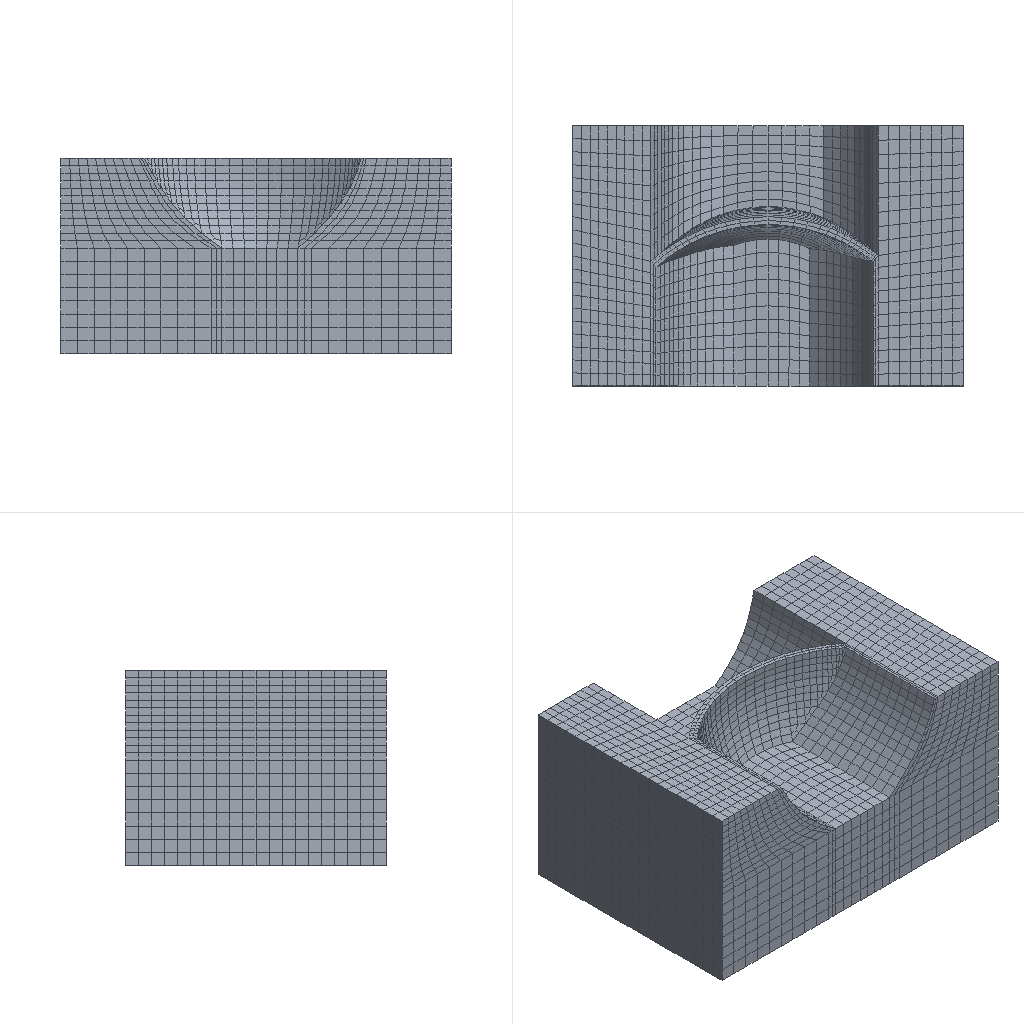Simulation study | abaqus
Set-up summary:
category,name,step,type,value,unit,region
solver,abaqus
solver,version,,,Abaqus/Standard 2020
units,not stated in the deck,,not stated
analysis,deck,,static,static
load_step,Step-2,Step-2,static
load_step,requested,,,1
mesh,nodes,,,11349
mesh,elements,,,9392
element_type,C3D8RP,,solid,9392
load,load commands in deck,,count,275
bc,support commands in deck,,count,1
material,MAT-BAJI,,in results
material,MAT-BATI,,in results
check,setup vs results,,match,"per instance, exact: element labels, types and connectivity; labels of the nodes the elements use; coordinates of those nodes at SINGLE_PRECISION in 1 of 1 instance(s)"
Abaqus input file, long lists of numbers shortened:
*Heading
** Job name: Job-2 Model name: model-mesh-Copy
** Generated by: Abaqus/CAE 2020
*Preprint, echo=NO, model=NO, history=NO, contact=NO
**
** PARTS
**
*Part, name=Part-10
*Node
      1,  -79.508,  -35.548,         57.5
      2,  -80.694,  -34.215,          69.
** (11347 more lines like these left out)
*Element, type=C3D8RP
1, 1819,  221, 1818, 6648,  219,    1,  220, 1817
2, 1818,  223, 1820, 6648,  220,    2,  222, 1817
** (9390 more lines like these left out)
*Nset, nset=bati
     1,     2,     3,     4,     5,     6,     7,     8,     9,    10,    11,    12,    13,    14,    15,    16
    17,    18,    19,    20,    21,    22,    23,    24,    25,    26,    27,    28,    29,    30,    31,    32
** (49 more lines like these left out)
*Elset, elset=bati
    1,    2,    3,    4,    5,    6,    7,    8,    9,   10,   11,   12,   13,   14,   15,   16
   17,   18,   19,   20,   21,   22,   23,   24,   25,   26,   27,   28,   29,   30,   31,   32
** (28 more lines like these left out)
*Nset, nset=baji
     1,     3,     5,     6,    15,    16,    26,    27,    38,    39,    52,    53,    68,    69,    70,    71
    72,    74,    75,    77,    98,    99,   108,   109,   117,   118,   121,   124,   127,   128,   129,   130
** (663 more lines like these left out)
*Elset, elset=baji, generate
  469,  9380,     1
** Section: Sec-bati
*Solid Section, elset=bati, material=Mat-bati
,
** Section: Sec-baji
*Solid Section, elset=baji, material=Mat-baji
,
*End Part
**
*Part, name=crack
*End Part
**
**
** ASSEMBLY
**
*Assembly, name=Assembly
**
*Instance, name=Part-10-1, part=Part-10
*End Instance
**
*Instance, name=crack-1, part=crack
23.198,       4.068, 38.045
23.198,       4.068, 38.045, 23.198, 5.068, 38.045, 80.
*End Instance
**
*Nset, nset=Set-9, instance=Part-10-1
    4,    5,    6,    7,   10,   11,   14,   15,   17,   20,   21,   23,   24,   26,   29,   30
   33,   34,   37,   38,   40,   42,   45,   46,   48,   50,   52,   55,   56,   59,   60,   63
** (15 more lines like these left out)
*Elset, elset=Set-9, instance=Part-10-1
    4,    5,    6,    7,    9,   11,   13,   16,   18,   20,   22,   23,   24,   25,   29,   31
   33,   35,   37,   39,   41,   43,   45,   47,   49,   51,   53,   54,   55,   59,   61,   63
** (13 more lines like these left out)
*Nset, nset=Set-10, instance=Part-10-1
    1,    2,    3,    4,    6,    8,    9,   10,   12,   13,   14,   16,   18,   19,   22,   25
   27,   28,   29,   31,   32,   33,   35,   36,   39,   41,   43,   44,   47,   49,   51,   53
** (19 more lines like these left out)
*Elset, elset=Set-10, instance=Part-10-1
    1,    2,    3,    4,    6,    8,    9,   10,   12,   13,   14,   15,   17,   19,   20,   21
   22,   26,   27,   28,   30,   32,   34,   36,   38,   40,   42,   44,   46,   48,   50,   52
** (15 more lines like these left out)
*Nset, nset=Set-11, instance=Part-10-1
     1,     2,     3,     4,     5,     6,     7,     8,     9,    10,    11,    12,    13,    14,    15,    16
    17,    18,    19,    20,    21,    22,    23,    24,    25,    26,    27,    28,    29,    30,    31,    32
** (49 more lines like these left out)
*Elset, elset=Set-11, instance=Part-10-1
    1,    2,    3,    4,    5,    6,    7,    8,    9,   10,   11,   12,   13,   14,   15,   16
   17,   18,   19,   20,   21,   22,   23,   24,   25,   26,   27,   28,   29,   30,   31,   32
** (34 more lines like these left out)
*Nset, nset=Set-14, instance=Part-10-1
  131,  132,  133,  134,  136,  137,  138,  139,  140,  142,  143,  145,  146,  150,  152,  154
  157,  158,  576,  577,  578,  579,  580,  581,  582,  583,  584,  585,  586,  587,  588,  589
** (35 more lines like these left out)
*Elset, elset=Set-14, instance=Part-10-1
  700,  701,  702,  703,  704,  705,  706,  707,  708,  709,  710,  711,  712,  713,  714,  715
  716,  717,  718,  719,  720,  721,  722,  723,  724,  725,  726,  727,  728,  729,  730,  731
** (32 more lines like these left out)
*Nset, nset=Set-15, instance=Part-10-1
    4,    5,    6,    7,   10,   11,   14,   15,   17,   20,   21,   23,   24,   26,   29,   30
   33,   34,   37,   38,   40,   42,   45,   46,   48,   50,   52,   55,   56,   59,   60,   63
** (15 more lines like these left out)
*Elset, elset=Set-15, instance=Part-10-1
    4,    5,    6,    7,    9,   11,   13,   16,   18,   20,   22,   23,   24,   25,   29,   31
   33,   35,   37,   39,   41,   43,   45,   47,   49,   51,   53,   54,   55,   59,   61,   63
** (14 more lines like these left out)
*Nset, nset=_PickedSet157, internal, instance=Part-10-1, generate
     1,  11349,      1
*Elset, elset=_PickedSet157, internal, instance=Part-10-1, generate
    1,  9392,     1
*Elset, elset=_Surf-5_S3, internal, instance=Part-10-1
   4,   6,  94, 191, 192, 195, 196, 199, 200, 214, 255, 256, 259, 260, 263, 264
 267, 268, 373, 374, 377, 378, 393, 431, 432, 467
*Elset, elset=_Surf-5_S4, internal, instance=Part-10-1
   5,  16,  18,  20,  22,  95,  96, 215, 224, 226, 228, 230, 232, 234, 236, 238
 240, 242, 244, 246, 248, 250, 252, 254, 358, 360, 362, 364, 382, 384, 386, 388
** (1 more lines like these left out)
*Elset, elset=_Surf-5_S6, internal, instance=Part-10-1
    7,    9,   11,   13,   29,   31,   33,   35,   37,   39,   41,   43,   45,   47,   49,   51
   59,   61,   63,   65,   67,   69,   71,   73,   75,   77,   79,   81,   83,   85,   87,   89
** (7 more lines like these left out)
*Elset, elset=_Surf-5_S2, internal, instance=Part-10-1
  23,  24,  25,  53,  54,  55, 137, 138, 139, 216, 217, 218, 219, 351, 352, 353
 457, 458, 459
*Elset, elset=_Surf-5_S1, internal, instance=Part-10-1, generate
 343,  350,    1
*Elset, elset=_Surf-5_S5, internal, instance=Part-10-1
 443, 444, 447, 448
*Surface, type=ELEMENT, name=Surf-5
_Surf-5_S3, S3
_Surf-5_S4, S4
_Surf-5_S6, S6
_Surf-5_S2, S2
_Surf-5_S1, S1
_Surf-5_S5, S5
*Enrichment, name=Crack-1, type=PROPAGATION CRACK, elset=_PickedSet157
*End Assembly
*Amplitude, name=Amp-1
             0.,              0.,             10.,              1.
**
** MATERIALS
**
*Material, name=Mat-baji
*Density
2770.,
*Elastic
 2.55e+10, 0.32
*Expansion
 1e-05,
*Fluid Leakoff
 1e-14, 1e-14
*Gap Flow
 0.001,
*Permeability, specific=9800.
 5.26e-09, 0.01
*Material, name=Mat-bati
*Damage Initiation, criterion=MAXPS, position=CRACKTIP
 2.5e+06,
*Damage Evolution, type=DISPLACEMENT
1.,
*Damage Stabilization
1e-05
*Density
2400.,
*Elastic
 2.55e+10, 0.2
*Expansion
 1e-05,
*Fluid Leakoff
 1e-14, 1e-14
*Gap Flow
 0.001,
*Permeability, specific=9800.
 5.26e-09, 0.01
**
** INTERACTION PROPERTIES
**
*Surface Interaction, name=IntProp-1
1.,
*Initial Conditions, type=ENRICHMENT
Part-10-1.281, 1,Crack-1, 5.75, 9.091
Part-10-1.281, 2,Crack-1, 5.75, 6.537
Part-10-1.281, 3,Crack-1, 1e-06, -4.361
Part-10-1.281, 4,Crack-1, 1e-06, 0.4588
Part-10-1.281, 5,Crack-1, -5.75, -1.695
Part-10-1.281, 6,Crack-1, -5.75, -3.416
Part-10-1.281, 7,Crack-1, 1e-06, 0.
Part-10-1.281, 8,Crack-1, 1e-06, 0.3126
Part-10-1.277, 1,Crack-1, -5.75, -1.695
Part-10-1.277, 2,Crack-1, -5.75, -3.416
Part-10-1.277, 3,Crack-1, 1e-06, 0.
Part-10-1.277, 4,Crack-1, 1e-06, 0.3126
Part-10-1.277, 5,Crack-1, -10.983, -12.704
Part-10-1.277, 6,Crack-1, -11.835, -13.569
Part-10-1.277, 7,Crack-1, -10.798, -13.53
Part-10-1.277, 8,Crack-1, -10.039, -12.759
**
** BOUNDARY CONDITIONS
**
** Name: BC-1 Type: 对称/反对称/完全固定
*Boundary
Set-14, ENCASTRE
**
** PREDEFINED FIELDS
**
** Name: Predefined Field-3   Type: Temperature
*Initial Conditions, type=TEMPERATURE
Set-11, 20.
** Name: Predefined Field-4   Type: Void ratio
*Initial Conditions, TYPE=RATIO
Part-10-1.bati, 0.7
** Name: Predefined Field-5   Type: Void ratio
*Initial Conditions, TYPE=RATIO
Part-10-1.baji, 0.4
** Name: Predefined Field-6   Type: Pore pressure
*Initial Conditions, TYPE=PORE PRESSURE
Set-15, 100000.
** Name: Predefined Field-7   Type: Void ratio
*Initial Conditions, TYPE=RATIO
Part-10-1.bati, 0.6
**
** INTERACTIONS
**
** Interaction: Int-1
*Contact
*Contact Inclusions, ALL EXTERIOR
*Contact Property Assignment
 ,  , IntProp-1
** ----------------------------------------------------------------
**
** STEP: Step-2
**
*Step, name=Step-2, nlgeom=YES, inc=1000
*Static, stabilize=0.0002, allsdtol=0.05, continue=NO
0.01, 1., 1e-05, 1.
**
** LOADS
**
** Name: Load-2   Type: Pressure
*Dsload
Surf-5, HP, 676200., 69., 0.
** Name: Load-4   Type: Gravity
*Dload
, GRAV, 9.8, 0., 0., -1.
**
** PREDEFINED FIELDS
**
** Name: Predefined Field-1   Type: Temperature Using Field: T-shangyou
*Temperature
Part-10-1.4, 32.
Part-10-1.5, 28.667
Part-10-1.6, 32.
Part-10-1.7, 28.667
Part-10-1.10, 32.
Part-10-1.11, 28.667
Part-10-1.14, 32.
Part-10-1.15, 25.333
Part-10-1.17, 25.333
Part-10-1.20, 28.667
Part-10-1.21, 25.333
Part-10-1.23, 28.667
Part-10-1.24, 22.
Part-10-1.26, 22.
Part-10-1.29, 32.
Part-10-1.30, 28.667
Part-10-1.33, 32.
Part-10-1.34, 22.
Part-10-1.37, 25.333
Part-10-1.38, 18.667
Part-10-1.40, 18.667
Part-10-1.42, 25.333
Part-10-1.45, 28.667
Part-10-1.46, 22.
Part-10-1.48, 18.667
Part-10-1.50, 15.333
Part-10-1.52, 15.333
Part-10-1.55, 32.
Part-10-1.56, 28.667
Part-10-1.59, 32.
Part-10-1.60, 22.
Part-10-1.63, 25.333
Part-10-1.64, 18.667
Part-10-1.66, 15.333
Part-10-1.68, 12.
Part-10-1.70, 12.
Part-10-1.72, 12.
Part-10-1.73, 15.333
Part-10-1.74, 15.333
Part-10-1.79, 22.
** (232 more lines like these left out)
** Name: Predefined Field-2   Type: Temperature
*Temperature
Set-10, 1.
**
** INTERACTIONS
**
** Interaction: Int-2
*Enrichment Activation, name=Crack-1, activate=ON
**
** OUTPUT REQUESTS
**
*Restart, write, frequency=0
**
** FIELD OUTPUT: F-Output-2
**
*Output, field
*Node Output
CF, NT, PHILSM, PSILSM, RF, U, V
*Element Output, directions=YES
E, LE, MISES, PE, PEEQ, PEMAG, RD, S, SDEG, TEMP
*Contact Output
CDISP, CSTRESS
*Output, history, frequency=0
*End Step
Results summary:
result,step,,partial,increments=0 time=0.0/1.0
result,analysis,,,static
result,last_loadstep,,,1
result,primary field,,,U
result,reaction total,,FX,0.0,model units
result,reaction total,,FY,0.0,model units
result,reaction total,,FZ,0.0,model units